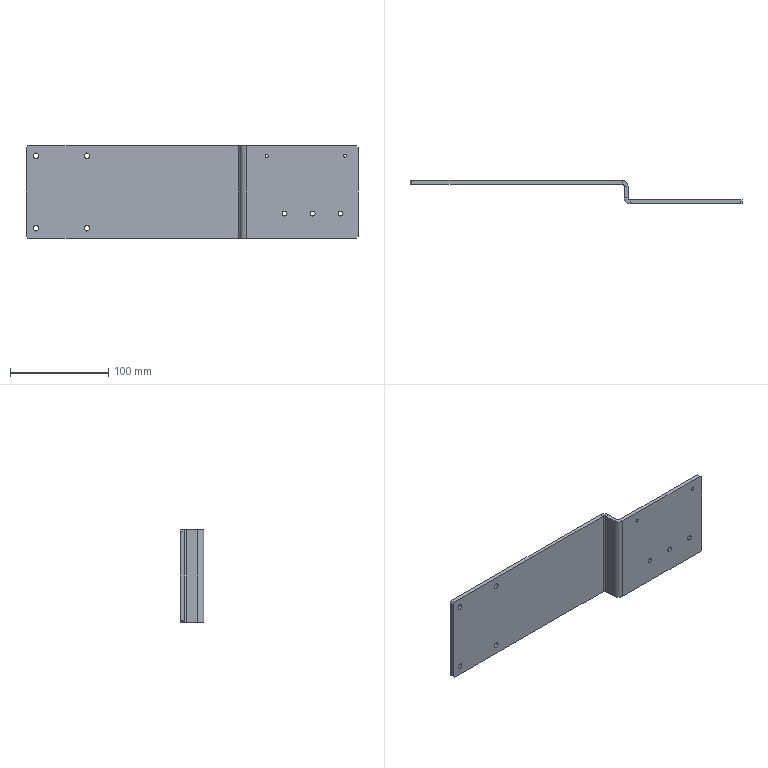Part | NX | features BREP 1 | 1 solid | 44 faces | box 338 x 24 x 94 mm | volume 132601 mm3 | cylinder 22 | plane 22 | commonest cylinder face diameters 5.5 x8 5 x6 3.3 x4 4 x2 12 x2
STEP:
#1=CARTESIAN_POINT('',(325.,-16.,35.35));
#2=VERTEX_POINT('',#1);
#3=CARTESIAN_POINT('',(325.,-20.,35.35));
#4=VERTEX_POINT('',#3);
#5=CARTESIAN_POINT('',(325.,-16.,35.35));
#6=DIRECTION('',(0.,1.,0.));
#7=VECTOR('',#6,1000.);
#8=LINE('',#5,#7);
#9=EDGE_CURVE('',#2,#4,#8,.F.);
#10=ORIENTED_EDGE('',*,*,#9,.T.);
#11=CARTESIAN_POINT('',(325.,-20.,38.65));
#12=VERTEX_POINT('',#11);
#13=CARTESIAN_POINT('',(325.,-20.,37.));
#14=DIRECTION('',(0.,1.,0.));
#15=DIRECTION('',(0.,0.,1.));
#16=AXIS2_PLACEMENT_3D('',#13,#14,#15);
#17=CIRCLE('',#16,1.65);
#18=EDGE_CURVE('',#12,#4,#17,.T.);
#19=ORIENTED_EDGE('',*,*,#18,.F.);
#20=CARTESIAN_POINT('',(325.,-16.,38.65));
#21=VERTEX_POINT('',#20);
#22=CARTESIAN_POINT('',(325.,-16.,38.65));
#23=DIRECTION('',(0.,1.,0.));
#24=VECTOR('',#23,1000.);
#25=LINE('',#22,#24);
#26=EDGE_CURVE('',#21,#12,#25,.F.);
#27=ORIENTED_EDGE('',*,*,#26,.F.);
#28=CARTESIAN_POINT('',(325.,-16.,37.));
#29=DIRECTION('',(0.,1.,0.));
#30=DIRECTION('',(0.,0.,1.));
#31=AXIS2_PLACEMENT_3D('',#28,#29,#30);
#32=CIRCLE('',#31,1.65);
#33=EDGE_CURVE('',#21,#2,#32,.T.);
#34=ORIENTED_EDGE('',*,*,#33,.T.);
#35=EDGE_LOOP('',(#10,#19,#27,#34));
#36=FACE_BOUND('',#35,.T.);
#37=CARTESIAN_POINT('',(325.,-16.,37.));
#38=DIRECTION('',(0.,1.,0.));
#39=DIRECTION('',(0.,0.,1.));
#40=AXIS2_PLACEMENT_3D('',#37,#38,#39);
#41=CYLINDRICAL_SURFACE('',#40,1.65);
#42=ADVANCED_FACE('',(#36),#41,.F.);
#43=CARTESIAN_POINT('',(245.,-16.,35.35));
#44=VERTEX_POINT('',#43);
#45=CARTESIAN_POINT('',(245.,-20.,35.35));
#46=VERTEX_POINT('',#45);
#47=CARTESIAN_POINT('',(245.,-16.,35.35));
#48=DIRECTION('',(0.,1.,0.));
#49=VECTOR('',#48,1000.);
#50=LINE('',#47,#49);
#51=EDGE_CURVE('',#44,#46,#50,.F.);
#52=ORIENTED_EDGE('',*,*,#51,.T.);
#53=CARTESIAN_POINT('',(245.,-20.,38.65));
#54=VERTEX_POINT('',#53);
#55=CARTESIAN_POINT('',(245.,-20.,37.));
#56=DIRECTION('',(0.,1.,0.));
#57=DIRECTION('',(0.,0.,1.));
#58=AXIS2_PLACEMENT_3D('',#55,#56,#57);
#59=CIRCLE('',#58,1.65);
#60=EDGE_CURVE('',#54,#46,#59,.T.);
#61=ORIENTED_EDGE('',*,*,#60,.F.);
#62=CARTESIAN_POINT('',(245.,-16.,38.65));
#63=VERTEX_POINT('',#62);
#64=CARTESIAN_POINT('',(245.,-16.,38.65));
#65=DIRECTION('',(0.,1.,0.));
#66=VECTOR('',#65,1000.);
#67=LINE('',#64,#66);
#68=EDGE_CURVE('',#63,#54,#67,.F.);
#69=ORIENTED_EDGE('',*,*,#68,.F.);
#70=CARTESIAN_POINT('',(245.,-16.,37.));
#71=DIRECTION('',(0.,1.,0.));
#72=DIRECTION('',(0.,0.,1.));
#73=AXIS2_PLACEMENT_3D('',#70,#71,#72);
#74=CIRCLE('',#73,1.65);
#75=EDGE_CURVE('',#63,#44,#74,.T.);
#76=ORIENTED_EDGE('',*,*,#75,.T.);
#77=EDGE_LOOP('',(#52,#61,#69,#76));
#78=FACE_BOUND('',#77,.T.);
#79=CARTESIAN_POINT('',(245.,-16.,37.));
#80=DIRECTION('',(0.,1.,0.));
#81=DIRECTION('',(0.,0.,1.));
#82=AXIS2_PLACEMENT_3D('',#79,#80,#81);
#83=CYLINDRICAL_SURFACE('',#82,1.65);
#84=ADVANCED_FACE('',(#78),#83,.F.);
#85=CARTESIAN_POINT('',(336.,-16.,47.));
#86=VERTEX_POINT('',#85);
#87=CARTESIAN_POINT('',(338.,-16.,45.));
#88=VERTEX_POINT('',#87);
#89=CARTESIAN_POINT('',(277.,-16.,106.));
#90=DIRECTION('',(0.7071,0.,-0.7071));
#91=VECTOR('',#90,1000.);
#92=LINE('',#89,#91);
#93=EDGE_CURVE('',#86,#88,#92,.T.);
#94=ORIENTED_EDGE('',*,*,#93,.F.);
#95=CARTESIAN_POINT('',(336.,-20.,47.));
#96=VERTEX_POINT('',#95);
#97=CARTESIAN_POINT('',(336.,-14.,47.));
#98=DIRECTION('',(0.,1.,0.));
#99=VECTOR('',#98,1000.);
#100=LINE('',#97,#99);
#101=EDGE_CURVE('',#96,#86,#100,.T.);
#102=ORIENTED_EDGE('',*,*,#101,.F.);
#103=CARTESIAN_POINT('',(338.,-20.,45.));
#104=VERTEX_POINT('',#103);
#105=CARTESIAN_POINT('',(338.,-20.,45.));
#106=DIRECTION('',(-0.7071,0.,0.7071));
#107=VECTOR('',#106,1000.);
#108=LINE('',#105,#107);
#109=EDGE_CURVE('',#104,#96,#108,.T.);
#110=ORIENTED_EDGE('',*,*,#109,.F.);
#111=CARTESIAN_POINT('',(338.,-16.,45.));
#112=DIRECTION('',(0.,-1.,0.));
#113=VECTOR('',#112,1000.);
#114=LINE('',#111,#113);
#115=EDGE_CURVE('',#88,#104,#114,.T.);
#116=ORIENTED_EDGE('',*,*,#115,.F.);
#117=EDGE_LOOP('',(#94,#102,#110,#116));
#118=FACE_BOUND('',#117,.T.);
#119=CARTESIAN_POINT('',(338.,-16.,45.));
#120=DIRECTION('',(-0.7071,0.,-0.7071));
#121=DIRECTION('',(0.,-1.,0.));
#122=AXIS2_PLACEMENT_3D('',#119,#120,#121);
#123=PLANE('',#122);
#124=ADVANCED_FACE('',(#118),#123,.F.);
#125=CARTESIAN_POINT('',(338.,-16.,-45.));
#126=VERTEX_POINT('',#125);
#127=CARTESIAN_POINT('',(336.,-16.,-47.));
#128=VERTEX_POINT('',#127);
#129=CARTESIAN_POINT('',(324.,-16.,-59.));
#130=DIRECTION('',(-0.7071,0.,-0.7071));
#131=VECTOR('',#130,1000.);
#132=LINE('',#129,#131);
#133=EDGE_CURVE('',#126,#128,#132,.T.);
#134=ORIENTED_EDGE('',*,*,#133,.F.);
#135=CARTESIAN_POINT('',(338.,-20.,-45.));
#136=VERTEX_POINT('',#135);
#137=CARTESIAN_POINT('',(338.,-16.,-45.));
#138=DIRECTION('',(0.,1.,0.));
#139=VECTOR('',#138,1000.);
#140=LINE('',#137,#139);
#141=EDGE_CURVE('',#136,#126,#140,.T.);
#142=ORIENTED_EDGE('',*,*,#141,.F.);
#143=CARTESIAN_POINT('',(336.,-20.,-47.));
#144=VERTEX_POINT('',#143);
#145=CARTESIAN_POINT('',(336.,-20.,-47.));
#146=DIRECTION('',(0.7071,0.,0.7071));
#147=VECTOR('',#146,1000.);
#148=LINE('',#145,#147);
#149=EDGE_CURVE('',#144,#136,#148,.T.);
#150=ORIENTED_EDGE('',*,*,#149,.F.);
#151=CARTESIAN_POINT('',(336.,-14.,-47.));
#152=DIRECTION('',(0.,-1.,0.));
#153=VECTOR('',#152,1000.);
#154=LINE('',#151,#153);
#155=EDGE_CURVE('',#128,#144,#154,.T.);
#156=ORIENTED_EDGE('',*,*,#155,.F.);
#157=EDGE_LOOP('',(#134,#142,#150,#156));
#158=FACE_BOUND('',#157,.T.);
#159=CARTESIAN_POINT('',(336.,-14.,-47.));
#160=DIRECTION('',(-0.7071,0.,0.7071));
#161=DIRECTION('',(0.,-1.,0.));
#162=AXIS2_PLACEMENT_3D('',#159,#160,#161);
#163=PLANE('',#162);
#164=ADVANCED_FACE('',(#158),#163,.F.);
#165=CARTESIAN_POINT('',(2.,0.,47.));
#166=VERTEX_POINT('',#165);
#167=CARTESIAN_POINT('',(0.,0.,45.));
#168=VERTEX_POINT('',#167);
#169=CARTESIAN_POINT('',(0.,0.,45.));
#170=DIRECTION('',(-0.7071,0.,-0.7071));
#171=VECTOR('',#170,1000.);
#172=LINE('',#169,#171);
#173=EDGE_CURVE('',#166,#168,#172,.T.);
#174=ORIENTED_EDGE('',*,*,#173,.F.);
#175=CARTESIAN_POINT('',(2.,4.,47.));
#176=VERTEX_POINT('',#175);
#177=CARTESIAN_POINT('',(2.,-2.,47.));
#178=DIRECTION('',(0.,-1.,0.));
#179=VECTOR('',#178,1000.);
#180=LINE('',#177,#179);
#181=EDGE_CURVE('',#176,#166,#180,.T.);
#182=ORIENTED_EDGE('',*,*,#181,.F.);
#183=CARTESIAN_POINT('',(0.,4.,45.));
#184=VERTEX_POINT('',#183);
#185=CARTESIAN_POINT('',(1.,4.,46.));
#186=DIRECTION('',(0.7071,0.,0.7071));
#187=VECTOR('',#186,1000.);
#188=LINE('',#185,#187);
#189=EDGE_CURVE('',#184,#176,#188,.T.);
#190=ORIENTED_EDGE('',*,*,#189,.F.);
#191=CARTESIAN_POINT('',(0.,0.,45.));
#192=DIRECTION('',(0.,1.,0.));
#193=VECTOR('',#192,1000.);
#194=LINE('',#191,#193);
#195=EDGE_CURVE('',#168,#184,#194,.T.);
#196=ORIENTED_EDGE('',*,*,#195,.F.);
#197=EDGE_LOOP('',(#174,#182,#190,#196));
#198=FACE_BOUND('',#197,.T.);
#199=CARTESIAN_POINT('',(0.,0.,45.));
#200=DIRECTION('',(0.7071,0.,-0.7071));
#201=DIRECTION('',(0.,1.,0.));
#202=AXIS2_PLACEMENT_3D('',#199,#200,#201);
#203=PLANE('',#202);
#204=ADVANCED_FACE('',(#198),#203,.F.);
#205=CARTESIAN_POINT('',(0.,0.,-45.));
#206=VERTEX_POINT('',#205);
#207=CARTESIAN_POINT('',(2.,0.,-47.));
#208=VERTEX_POINT('',#207);
#209=CARTESIAN_POINT('',(2.,0.,-47.));
#210=DIRECTION('',(0.7071,0.,-0.7071));
#211=VECTOR('',#210,1000.);
#212=LINE('',#209,#211);
#213=EDGE_CURVE('',#206,#208,#212,.T.);
#214=ORIENTED_EDGE('',*,*,#213,.F.);
#215=CARTESIAN_POINT('',(0.,4.,-45.));
#216=VERTEX_POINT('',#215);
#217=CARTESIAN_POINT('',(0.,0.,-45.));
#218=DIRECTION('',(0.,-1.,0.));
#219=VECTOR('',#218,1000.);
#220=LINE('',#217,#219);
#221=EDGE_CURVE('',#216,#206,#220,.T.);
#222=ORIENTED_EDGE('',*,*,#221,.F.);
#223=CARTESIAN_POINT('',(2.,4.,-47.));
#224=VERTEX_POINT('',#223);
#225=CARTESIAN_POINT('',(-46.,4.,1.));
#226=DIRECTION('',(-0.7071,0.,0.7071));
#227=VECTOR('',#226,1000.);
#228=LINE('',#225,#227);
#229=EDGE_CURVE('',#224,#216,#228,.T.);
#230=ORIENTED_EDGE('',*,*,#229,.F.);
#231=CARTESIAN_POINT('',(2.,4.,-47.));
#232=DIRECTION('',(0.,1.,0.));
#233=VECTOR('',#232,1000.);
#234=LINE('',#231,#233);
#235=EDGE_CURVE('',#208,#224,#234,.T.);
#236=ORIENTED_EDGE('',*,*,#235,.F.);
#237=EDGE_LOOP('',(#214,#222,#230,#236));
#238=FACE_BOUND('',#237,.T.);
#239=CARTESIAN_POINT('',(2.,-14.,-47.));
#240=DIRECTION('',(-0.7071,0.,-0.7071));
#241=DIRECTION('',(0.,-1.,0.));
#242=AXIS2_PLACEMENT_3D('',#239,#240,#241);
#243=PLANE('',#242);
#244=ADVANCED_FACE('',(#238),#243,.T.);
#245=CARTESIAN_POINT('',(263.3,-16.,-24.5));
#246=VERTEX_POINT('',#245);
#247=CARTESIAN_POINT('',(263.3,-20.,-24.5));
#248=VERTEX_POINT('',#247);
#249=CARTESIAN_POINT('',(263.3,-16.,-24.5));
#250=DIRECTION('',(0.,1.,0.));
#251=VECTOR('',#250,1000.);
#252=LINE('',#249,#251);
#253=EDGE_CURVE('',#246,#248,#252,.F.);
#254=ORIENTED_EDGE('',*,*,#253,.T.);
#255=CARTESIAN_POINT('',(263.3,-20.,-19.5));
#256=VERTEX_POINT('',#255);
#257=CARTESIAN_POINT('',(263.3,-20.,-22.));
#258=DIRECTION('',(0.,1.,0.));
#259=DIRECTION('',(0.,0.,1.));
#260=AXIS2_PLACEMENT_3D('',#257,#258,#259);
#261=CIRCLE('',#260,2.5);
#262=EDGE_CURVE('',#256,#248,#261,.T.);
#263=ORIENTED_EDGE('',*,*,#262,.F.);
#264=CARTESIAN_POINT('',(263.3,-16.,-19.5));
#265=VERTEX_POINT('',#264);
#266=CARTESIAN_POINT('',(263.3,-16.,-19.5));
#267=DIRECTION('',(0.,1.,0.));
#268=VECTOR('',#267,1000.);
#269=LINE('',#266,#268);
#270=EDGE_CURVE('',#265,#256,#269,.F.);
#271=ORIENTED_EDGE('',*,*,#270,.F.);
#272=CARTESIAN_POINT('',(263.3,-16.,-22.));
#273=DIRECTION('',(0.,1.,0.));
#274=DIRECTION('',(0.,0.,1.));
#275=AXIS2_PLACEMENT_3D('',#272,#273,#274);
#276=CIRCLE('',#275,2.5);
#277=EDGE_CURVE('',#265,#246,#276,.T.);
#278=ORIENTED_EDGE('',*,*,#277,.T.);
#279=EDGE_LOOP('',(#254,#263,#271,#278));
#280=FACE_BOUND('',#279,.T.);
#281=CARTESIAN_POINT('',(263.3,-16.,-22.));
#282=DIRECTION('',(0.,1.,0.));
#283=DIRECTION('',(0.,0.,1.));
#284=AXIS2_PLACEMENT_3D('',#281,#282,#283);
#285=CYLINDRICAL_SURFACE('',#284,2.5);
#286=ADVANCED_FACE('',(#280),#285,.F.);
#287=CARTESIAN_POINT('',(291.8,-16.,-24.5));
#288=VERTEX_POINT('',#287);
#289=CARTESIAN_POINT('',(291.8,-20.,-24.5));
#290=VERTEX_POINT('',#289);
#291=CARTESIAN_POINT('',(291.8,-16.,-24.5));
#292=DIRECTION('',(0.,1.,0.));
#293=VECTOR('',#292,1000.);
#294=LINE('',#291,#293);
#295=EDGE_CURVE('',#288,#290,#294,.F.);
#296=ORIENTED_EDGE('',*,*,#295,.T.);
#297=CARTESIAN_POINT('',(291.8,-20.,-19.5));
#298=VERTEX_POINT('',#297);
#299=CARTESIAN_POINT('',(291.8,-20.,-22.));
#300=DIRECTION('',(0.,1.,0.));
#301=DIRECTION('',(0.,0.,1.));
#302=AXIS2_PLACEMENT_3D('',#299,#300,#301);
#303=CIRCLE('',#302,2.5);
#304=EDGE_CURVE('',#298,#290,#303,.T.);
#305=ORIENTED_EDGE('',*,*,#304,.F.);
#306=CARTESIAN_POINT('',(291.8,-16.,-19.5));
#307=VERTEX_POINT('',#306);
#308=CARTESIAN_POINT('',(291.8,-16.,-19.5));
#309=DIRECTION('',(0.,1.,0.));
#310=VECTOR('',#309,1000.);
#311=LINE('',#308,#310);
#312=EDGE_CURVE('',#307,#298,#311,.F.);
#313=ORIENTED_EDGE('',*,*,#312,.F.);
#314=CARTESIAN_POINT('',(291.8,-16.,-22.));
#315=DIRECTION('',(0.,1.,0.));
#316=DIRECTION('',(0.,0.,1.));
#317=AXIS2_PLACEMENT_3D('',#314,#315,#316);
#318=CIRCLE('',#317,2.5);
#319=EDGE_CURVE('',#307,#288,#318,.T.);
#320=ORIENTED_EDGE('',*,*,#319,.T.);
#321=EDGE_LOOP('',(#296,#305,#313,#320));
#322=FACE_BOUND('',#321,.T.);
#323=CARTESIAN_POINT('',(291.8,-16.,-22.));
#324=DIRECTION('',(0.,1.,0.));
#325=DIRECTION('',(0.,0.,1.));
#326=AXIS2_PLACEMENT_3D('',#323,#324,#325);
#327=CYLINDRICAL_SURFACE('',#326,2.5);
#328=ADVANCED_FACE('',(#322),#327,.F.);
#329=CARTESIAN_POINT('',(320.3,-16.,-24.5));
#330=VERTEX_POINT('',#329);
#331=CARTESIAN_POINT('',(320.3,-20.,-24.5));
#332=VERTEX_POINT('',#331);
#333=CARTESIAN_POINT('',(320.3,-16.,-24.5));
#334=DIRECTION('',(0.,1.,0.));
#335=VECTOR('',#334,1000.);
#336=LINE('',#333,#335);
#337=EDGE_CURVE('',#330,#332,#336,.F.);
#338=ORIENTED_EDGE('',*,*,#337,.T.);
#339=CARTESIAN_POINT('',(320.3,-20.,-19.5));
#340=VERTEX_POINT('',#339);
#341=CARTESIAN_POINT('',(320.3,-20.,-22.));
#342=DIRECTION('',(0.,1.,0.));
#343=DIRECTION('',(0.,0.,1.));
#344=AXIS2_PLACEMENT_3D('',#341,#342,#343);
#345=CIRCLE('',#344,2.5);
#346=EDGE_CURVE('',#340,#332,#345,.T.);
#347=ORIENTED_EDGE('',*,*,#346,.F.);
#348=CARTESIAN_POINT('',(320.3,-16.,-19.5));
#349=VERTEX_POINT('',#348);
#350=CARTESIAN_POINT('',(320.3,-16.,-19.5));
#351=DIRECTION('',(0.,1.,0.));
#352=VECTOR('',#351,1000.);
#353=LINE('',#350,#352);
#354=EDGE_CURVE('',#349,#340,#353,.F.);
#355=ORIENTED_EDGE('',*,*,#354,.F.);
#356=CARTESIAN_POINT('',(320.3,-16.,-22.));
#357=DIRECTION('',(0.,1.,0.));
#358=DIRECTION('',(0.,0.,1.));
#359=AXIS2_PLACEMENT_3D('',#356,#357,#358);
#360=CIRCLE('',#359,2.5);
#361=EDGE_CURVE('',#349,#330,#360,.T.);
#362=ORIENTED_EDGE('',*,*,#361,.T.);
#363=EDGE_LOOP('',(#338,#347,#355,#362));
#364=FACE_BOUND('',#363,.T.);
#365=CARTESIAN_POINT('',(320.3,-16.,-22.));
#366=DIRECTION('',(0.,1.,0.));
#367=DIRECTION('',(0.,0.,1.));
#368=AXIS2_PLACEMENT_3D('',#365,#366,#367);
#369=CYLINDRICAL_SURFACE('',#368,2.5);
#370=ADVANCED_FACE('',(#364),#369,.F.);
#371=CARTESIAN_POINT('',(10.,4.,-39.75));
#372=VERTEX_POINT('',#371);
#373=CARTESIAN_POINT('',(10.,0.,-39.75));
#374=VERTEX_POINT('',#373);
#375=CARTESIAN_POINT('',(10.,4.,-39.75));
#376=DIRECTION('',(0.,1.,0.));
#377=VECTOR('',#376,1000.);
#378=LINE('',#375,#377);
#379=EDGE_CURVE('',#372,#374,#378,.F.);
#380=ORIENTED_EDGE('',*,*,#379,.T.);
#381=CARTESIAN_POINT('',(10.,0.,-34.25));
#382=VERTEX_POINT('',#381);
#383=CARTESIAN_POINT('',(10.,0.,-37.));
#384=DIRECTION('',(0.,1.,0.));
#385=DIRECTION('',(0.,0.,1.));
#386=AXIS2_PLACEMENT_3D('',#383,#384,#385);
#387=CIRCLE('',#386,2.75);
#388=EDGE_CURVE('',#382,#374,#387,.T.);
#389=ORIENTED_EDGE('',*,*,#388,.F.);
#390=CARTESIAN_POINT('',(10.,4.,-34.25));
#391=VERTEX_POINT('',#390);
#392=CARTESIAN_POINT('',(10.,4.,-34.25));
#393=DIRECTION('',(0.,1.,0.));
#394=VECTOR('',#393,1000.);
#395=LINE('',#392,#394);
#396=EDGE_CURVE('',#391,#382,#395,.F.);
#397=ORIENTED_EDGE('',*,*,#396,.F.);
#398=CARTESIAN_POINT('',(10.,4.,-37.));
#399=DIRECTION('',(0.,1.,0.));
#400=DIRECTION('',(0.,0.,1.));
#401=AXIS2_PLACEMENT_3D('',#398,#399,#400);
#402=CIRCLE('',#401,2.75);
#403=EDGE_CURVE('',#391,#372,#402,.T.);
#404=ORIENTED_EDGE('',*,*,#403,.T.);
#405=EDGE_LOOP('',(#380,#389,#397,#404));
#406=FACE_BOUND('',#405,.T.);
#407=CARTESIAN_POINT('',(10.,4.,-37.));
#408=DIRECTION('',(0.,1.,0.));
#409=DIRECTION('',(0.,0.,1.));
#410=AXIS2_PLACEMENT_3D('',#407,#408,#409);
#411=CYLINDRICAL_SURFACE('',#410,2.75);
#412=ADVANCED_FACE('',(#406),#411,.F.);
#413=CARTESIAN_POINT('',(62.,4.,-39.75));
#414=VERTEX_POINT('',#413);
#415=CARTESIAN_POINT('',(62.,0.,-39.75));
#416=VERTEX_POINT('',#415);
#417=CARTESIAN_POINT('',(62.,4.,-39.75));
#418=DIRECTION('',(0.,1.,0.));
#419=VECTOR('',#418,1000.);
#420=LINE('',#417,#419);
#421=EDGE_CURVE('',#414,#416,#420,.F.);
#422=ORIENTED_EDGE('',*,*,#421,.T.);
#423=CARTESIAN_POINT('',(62.,0.,-34.25));
#424=VERTEX_POINT('',#423);
#425=CARTESIAN_POINT('',(62.,0.,-37.));
#426=DIRECTION('',(0.,1.,0.));
#427=DIRECTION('',(0.,0.,1.));
#428=AXIS2_PLACEMENT_3D('',#425,#426,#427);
#429=CIRCLE('',#428,2.75);
#430=EDGE_CURVE('',#424,#416,#429,.T.);
#431=ORIENTED_EDGE('',*,*,#430,.F.);
#432=CARTESIAN_POINT('',(62.,4.,-34.25));
#433=VERTEX_POINT('',#432);
#434=CARTESIAN_POINT('',(62.,4.,-34.25));
#435=DIRECTION('',(0.,1.,0.));
#436=VECTOR('',#435,1000.);
#437=LINE('',#434,#436);
#438=EDGE_CURVE('',#433,#424,#437,.F.);
#439=ORIENTED_EDGE('',*,*,#438,.F.);
#440=CARTESIAN_POINT('',(62.,4.,-37.));
#441=DIRECTION('',(0.,1.,0.));
#442=DIRECTION('',(0.,0.,1.));
#443=AXIS2_PLACEMENT_3D('',#440,#441,#442);
#444=CIRCLE('',#443,2.75);
#445=EDGE_CURVE('',#433,#414,#444,.T.);
#446=ORIENTED_EDGE('',*,*,#445,.T.);
#447=EDGE_LOOP('',(#422,#431,#439,#446));
#448=FACE_BOUND('',#447,.T.);
#449=CARTESIAN_POINT('',(62.,4.,-37.));
#450=DIRECTION('',(0.,1.,0.));
#451=DIRECTION('',(0.,0.,1.));
#452=AXIS2_PLACEMENT_3D('',#449,#450,#451);
#453=CYLINDRICAL_SURFACE('',#452,2.75);
#454=ADVANCED_FACE('',(#448),#453,.F.);
#455=CARTESIAN_POINT('',(10.,4.,34.25));
#456=VERTEX_POINT('',#455);
#457=CARTESIAN_POINT('',(10.,0.,34.25));
#458=VERTEX_POINT('',#457);
#459=CARTESIAN_POINT('',(10.,4.,34.25));
#460=DIRECTION('',(0.,1.,0.));
#461=VECTOR('',#460,1000.);
#462=LINE('',#459,#461);
#463=EDGE_CURVE('',#456,#458,#462,.F.);
#464=ORIENTED_EDGE('',*,*,#463,.T.);
#465=CARTESIAN_POINT('',(10.,0.,39.75));
#466=VERTEX_POINT('',#465);
#467=CARTESIAN_POINT('',(10.,0.,37.));
#468=DIRECTION('',(0.,1.,0.));
#469=DIRECTION('',(0.,0.,1.));
#470=AXIS2_PLACEMENT_3D('',#467,#468,#469);
#471=CIRCLE('',#470,2.75);
#472=EDGE_CURVE('',#466,#458,#471,.T.);
#473=ORIENTED_EDGE('',*,*,#472,.F.);
#474=CARTESIAN_POINT('',(10.,4.,39.75));
#475=VERTEX_POINT('',#474);
#476=CARTESIAN_POINT('',(10.,4.,39.75));
#477=DIRECTION('',(0.,1.,0.));
#478=VECTOR('',#477,1000.);
#479=LINE('',#476,#478);
#480=EDGE_CURVE('',#475,#466,#479,.F.);
#481=ORIENTED_EDGE('',*,*,#480,.F.);
#482=CARTESIAN_POINT('',(10.,4.,37.));
#483=DIRECTION('',(0.,1.,0.));
#484=DIRECTION('',(0.,0.,1.));
#485=AXIS2_PLACEMENT_3D('',#482,#483,#484);
#486=CIRCLE('',#485,2.75);
#487=EDGE_CURVE('',#475,#456,#486,.T.);
#488=ORIENTED_EDGE('',*,*,#487,.T.);
#489=EDGE_LOOP('',(#464,#473,#481,#488));
#490=FACE_BOUND('',#489,.T.);
#491=CARTESIAN_POINT('',(10.,4.,37.));
#492=DIRECTION('',(0.,1.,0.));
#493=DIRECTION('',(0.,0.,1.));
#494=AXIS2_PLACEMENT_3D('',#491,#492,#493);
#495=CYLINDRICAL_SURFACE('',#494,2.75);
#496=ADVANCED_FACE('',(#490),#495,.F.);
#497=CARTESIAN_POINT('',(62.,4.,34.25));
#498=VERTEX_POINT('',#497);
#499=CARTESIAN_POINT('',(62.,0.,34.25));
#500=VERTEX_POINT('',#499);
#501=CARTESIAN_POINT('',(62.,4.,34.25));
#502=DIRECTION('',(0.,1.,0.));
#503=VECTOR('',#502,1000.);
#504=LINE('',#501,#503);
#505=EDGE_CURVE('',#498,#500,#504,.F.);
#506=ORIENTED_EDGE('',*,*,#505,.T.);
#507=CARTESIAN_POINT('',(62.,0.,39.75));
#508=VERTEX_POINT('',#507);
#509=CARTESIAN_POINT('',(62.,0.,37.));
#510=DIRECTION('',(0.,1.,0.));
#511=DIRECTION('',(0.,0.,1.));
#512=AXIS2_PLACEMENT_3D('',#509,#510,#511);
#513=CIRCLE('',#512,2.75);
#514=EDGE_CURVE('',#508,#500,#513,.T.);
#515=ORIENTED_EDGE('',*,*,#514,.F.);
#516=CARTESIAN_POINT('',(62.,4.,39.75));
#517=VERTEX_POINT('',#516);
#518=CARTESIAN_POINT('',(62.,4.,39.75));
#519=DIRECTION('',(0.,1.,0.));
#520=VECTOR('',#519,1000.);
#521=LINE('',#518,#520);
#522=EDGE_CURVE('',#517,#508,#521,.F.);
#523=ORIENTED_EDGE('',*,*,#522,.F.);
#524=CARTESIAN_POINT('',(62.,4.,37.));
#525=DIRECTION('',(0.,1.,0.));
#526=DIRECTION('',(0.,0.,1.));
#527=AXIS2_PLACEMENT_3D('',#524,#525,#526);
#528=CIRCLE('',#527,2.75);
#529=EDGE_CURVE('',#517,#498,#528,.T.);
#530=ORIENTED_EDGE('',*,*,#529,.T.);
#531=EDGE_LOOP('',(#506,#515,#523,#530));
#532=FACE_BOUND('',#531,.T.);
#533=CARTESIAN_POINT('',(62.,4.,37.));
#534=DIRECTION('',(0.,1.,0.));
#535=DIRECTION('',(0.,0.,1.));
#536=AXIS2_PLACEMENT_3D('',#533,#534,#535);
#537=CYLINDRICAL_SURFACE('',#536,2.75);
#538=ADVANCED_FACE('',(#532),#537,.F.);
#539=CARTESIAN_POINT('',(216.,0.,-47.));
#540=VERTEX_POINT('',#539);
#541=CARTESIAN_POINT('',(0.,0.,-47.));
#542=DIRECTION('',(1.,0.,0.));
#543=VECTOR('',#542,1000.);
#544=LINE('',#541,#543);
#545=EDGE_CURVE('',#208,#540,#544,.T.);
#546=ORIENTED_EDGE('',*,*,#545,.F.);
#547=ORIENTED_EDGE('',*,*,#235,.T.);
#548=CARTESIAN_POINT('',(216.,4.,-47.));
#549=VERTEX_POINT('',#548);
#550=CARTESIAN_POINT('',(0.,4.,-47.));
#551=DIRECTION('',(1.,0.,0.));
#552=VECTOR('',#551,1000.);
#553=LINE('',#550,#552);
#554=EDGE_CURVE('',#224,#549,#553,.T.);
#555=ORIENTED_EDGE('',*,*,#554,.T.);
#556=CARTESIAN_POINT('',(216.,4.,-47.));
#557=DIRECTION('',(0.,-1.,0.));
#558=VECTOR('',#557,1000.);
#559=LINE('',#556,#558);
#560=EDGE_CURVE('',#549,#540,#559,.T.);
#561=ORIENTED_EDGE('',*,*,#560,.T.);
#562=EDGE_LOOP('',(#546,#547,#555,#561));
#563=FACE_BOUND('',#562,.T.);
#564=CARTESIAN_POINT('',(224.,-14.,-47.));
#565=DIRECTION('',(0.,0.,1.));
#566=DIRECTION('',(1.,0.,0.));
#567=AXIS2_PLACEMENT_3D('',#564,#565,#566);
#568=PLANE('',#567);
#569=ADVANCED_FACE('',(#563),#568,.F.);
#570=CARTESIAN_POINT('',(224.,-20.,47.));
#571=VERTEX_POINT('',#570);
#572=CARTESIAN_POINT('',(218.,-20.,47.));
#573=DIRECTION('',(1.,0.,0.));
#574=VECTOR('',#573,1000.);
#575=LINE('',#572,#574);
#576=EDGE_CURVE('',#571,#96,#575,.T.);
#577=ORIENTED_EDGE('',*,*,#576,.T.);
#578=ORIENTED_EDGE('',*,*,#101,.T.);
#579=CARTESIAN_POINT('',(224.,-16.,47.));
#580=VERTEX_POINT('',#579);
#581=CARTESIAN_POINT('',(218.,-16.,47.));
#582=DIRECTION('',(1.,0.,0.));
#583=VECTOR('',#582,1000.);
#584=LINE('',#581,#583);
#585=EDGE_CURVE('',#580,#86,#584,.T.);
#586=ORIENTED_EDGE('',*,*,#585,.F.);
#587=CARTESIAN_POINT('',(224.,-16.,47.));
#588=DIRECTION('',(0.,-1.,0.));
#589=VECTOR('',#588,1000.);
#590=LINE('',#587,#589);
#591=EDGE_CURVE('',#580,#571,#590,.T.);
#592=ORIENTED_EDGE('',*,*,#591,.T.);
#593=EDGE_LOOP('',(#577,#578,#586,#592));
#594=FACE_BOUND('',#593,.T.);
#595=CARTESIAN_POINT('',(224.,-14.,47.));
#596=DIRECTION('',(0.,0.,1.));
#597=DIRECTION('',(1.,0.,0.));
#598=AXIS2_PLACEMENT_3D('',#595,#596,#597);
#599=PLANE('',#598);
#600=ADVANCED_FACE('',(#594),#599,.T.);
#601=CARTESIAN_POINT('',(218.,-14.,-47.));
#602=VERTEX_POINT('',#601);
#603=CARTESIAN_POINT('',(224.,-20.,-47.));
#604=VERTEX_POINT('',#603);
#605=CARTESIAN_POINT('',(224.,-14.,-47.));
#606=DIRECTION('',(0.,0.,1.));
#607=DIRECTION('',(-1.,0.,0.));
#608=AXIS2_PLACEMENT_3D('',#605,#606,#607);
#609=CIRCLE('',#608,6.);
#610=EDGE_CURVE('',#602,#604,#609,.T.);
#611=ORIENTED_EDGE('',*,*,#610,.T.);
#612=CARTESIAN_POINT('',(224.,-20.,47.));
#613=DIRECTION('',(0.,0.,-1.));
#614=VECTOR('',#613,1000.);
#615=LINE('',#612,#614);
#616=EDGE_CURVE('',#571,#604,#615,.T.);
#617=ORIENTED_EDGE('',*,*,#616,.F.);
#618=CARTESIAN_POINT('',(218.,-14.,47.));
#619=VERTEX_POINT('',#618);
#620=CARTESIAN_POINT('',(224.,-14.,47.));
#621=DIRECTION('',(0.,0.,1.));
#622=DIRECTION('',(-1.,0.,0.));
#623=AXIS2_PLACEMENT_3D('',#620,#621,#622);
#624=CIRCLE('',#623,6.);
#625=EDGE_CURVE('',#619,#571,#624,.T.);
#626=ORIENTED_EDGE('',*,*,#625,.F.);
#627=CARTESIAN_POINT('',(218.,-14.,47.));
#628=DIRECTION('',(0.,0.,-1.));
#629=VECTOR('',#628,1000.);
#630=LINE('',#627,#629);
#631=EDGE_CURVE('',#619,#602,#630,.T.);
#632=ORIENTED_EDGE('',*,*,#631,.T.);
#633=EDGE_LOOP('',(#611,#617,#626,#632));
#634=FACE_BOUND('',#633,.T.);
#635=CARTESIAN_POINT('',(224.,-14.,47.));
#636=DIRECTION('',(0.,0.,-1.));
#637=DIRECTION('',(-1.,0.,0.));
#638=AXIS2_PLACEMENT_3D('',#635,#636,#637);
#639=CYLINDRICAL_SURFACE('',#638,6.);
#640=ADVANCED_FACE('',(#634),#639,.T.);
#641=CARTESIAN_POINT('',(218.,-2.,-47.));
#642=VERTEX_POINT('',#641);
#643=CARTESIAN_POINT('',(218.,0.,-47.));
#644=DIRECTION('',(0.,-1.,0.));
#645=VECTOR('',#644,1000.);
#646=LINE('',#643,#645);
#647=EDGE_CURVE('',#642,#602,#646,.T.);
#648=ORIENTED_EDGE('',*,*,#647,.T.);
#649=ORIENTED_EDGE('',*,*,#631,.F.);
#650=CARTESIAN_POINT('',(218.,-2.,47.));
#651=VERTEX_POINT('',#650);
#652=CARTESIAN_POINT('',(218.,0.,47.));
#653=DIRECTION('',(0.,-1.,0.));
#654=VECTOR('',#653,1000.);
#655=LINE('',#652,#654);
#656=EDGE_CURVE('',#651,#619,#655,.T.);
#657=ORIENTED_EDGE('',*,*,#656,.F.);
#658=CARTESIAN_POINT('',(218.,-2.,47.));
#659=DIRECTION('',(0.,0.,-1.));
#660=VECTOR('',#659,1000.);
#661=LINE('',#658,#660);
#662=EDGE_CURVE('',#651,#642,#661,.T.);
#663=ORIENTED_EDGE('',*,*,#662,.T.);
#664=EDGE_LOOP('',(#648,#649,#657,#663));
#665=FACE_BOUND('',#664,.T.);
#666=CARTESIAN_POINT('',(218.,0.,47.));
#667=DIRECTION('',(1.,0.,0.));
#668=DIRECTION('',(0.,0.,-1.));
#669=AXIS2_PLACEMENT_3D('',#666,#667,#668);
#670=PLANE('',#669);
#671=ADVANCED_FACE('',(#665),#670,.F.);
#672=CARTESIAN_POINT('',(216.,-2.,-47.));
#673=DIRECTION('',(0.,0.,-1.));
#674=DIRECTION('',(1.,0.,0.));
#675=AXIS2_PLACEMENT_3D('',#672,#673,#674);
#676=CIRCLE('',#675,2.);
#677=EDGE_CURVE('',#540,#642,#676,.T.);
#678=ORIENTED_EDGE('',*,*,#677,.T.);
#679=ORIENTED_EDGE('',*,*,#662,.F.);
#680=CARTESIAN_POINT('',(216.,0.,47.));
#681=VERTEX_POINT('',#680);
#682=CARTESIAN_POINT('',(216.,-2.,47.));
#683=DIRECTION('',(0.,0.,-1.));
#684=DIRECTION('',(1.,0.,0.));
#685=AXIS2_PLACEMENT_3D('',#682,#683,#684);
#686=CIRCLE('',#685,2.);
#687=EDGE_CURVE('',#681,#651,#686,.T.);
#688=ORIENTED_EDGE('',*,*,#687,.F.);
#689=CARTESIAN_POINT('',(216.,0.,47.));
#690=DIRECTION('',(0.,0.,-1.));
#691=VECTOR('',#690,1000.);
#692=LINE('',#689,#691);
#693=EDGE_CURVE('',#681,#540,#692,.T.);
#694=ORIENTED_EDGE('',*,*,#693,.T.);
#695=EDGE_LOOP('',(#678,#679,#688,#694));
#696=FACE_BOUND('',#695,.T.);
#697=CARTESIAN_POINT('',(216.,-2.,47.));
#698=DIRECTION('',(0.,0.,-1.));
#699=DIRECTION('',(-1.,0.,0.));
#700=AXIS2_PLACEMENT_3D('',#697,#698,#699);
#701=CYLINDRICAL_SURFACE('',#700,2.);
#702=ADVANCED_FACE('',(#696),#701,.F.);
#703=CARTESIAN_POINT('',(0.,0.,47.));
#704=DIRECTION('',(0.,0.,-1.));
#705=VECTOR('',#704,1000.);
#706=LINE('',#703,#705);
#707=EDGE_CURVE('',#168,#206,#706,.T.);
#708=ORIENTED_EDGE('',*,*,#707,.T.);
#709=ORIENTED_EDGE('',*,*,#213,.T.);
#710=ORIENTED_EDGE('',*,*,#545,.T.);
#711=ORIENTED_EDGE('',*,*,#693,.F.);
#712=CARTESIAN_POINT('',(0.,0.,47.));
#713=DIRECTION('',(1.,0.,0.));
#714=VECTOR('',#713,1000.);
#715=LINE('',#712,#714);
#716=EDGE_CURVE('',#166,#681,#715,.T.);
#717=ORIENTED_EDGE('',*,*,#716,.F.);
#718=ORIENTED_EDGE('',*,*,#173,.T.);
#719=EDGE_LOOP('',(#708,#709,#710,#711,#717,#718));
#720=FACE_BOUND('',#719,.T.);
#721=ORIENTED_EDGE('',*,*,#514,.T.);
#722=CARTESIAN_POINT('',(62.,0.,37.));
#723=DIRECTION('',(0.,1.,0.));
#724=DIRECTION('',(0.,0.,1.));
#725=AXIS2_PLACEMENT_3D('',#722,#723,#724);
#726=CIRCLE('',#725,2.75);
#727=EDGE_CURVE('',#500,#508,#726,.T.);
#728=ORIENTED_EDGE('',*,*,#727,.T.);
#729=EDGE_LOOP('',(#721,#728));
#730=FACE_BOUND('',#729,.T.);
#731=ORIENTED_EDGE('',*,*,#472,.T.);
#732=CARTESIAN_POINT('',(10.,0.,37.));
#733=DIRECTION('',(0.,1.,0.));
#734=DIRECTION('',(0.,0.,1.));
#735=AXIS2_PLACEMENT_3D('',#732,#733,#734);
#736=CIRCLE('',#735,2.75);
#737=EDGE_CURVE('',#458,#466,#736,.T.);
#738=ORIENTED_EDGE('',*,*,#737,.T.);
#739=EDGE_LOOP('',(#731,#738));
#740=FACE_BOUND('',#739,.T.);
#741=ORIENTED_EDGE('',*,*,#430,.T.);
#742=CARTESIAN_POINT('',(62.,0.,-37.));
#743=DIRECTION('',(0.,1.,0.));
#744=DIRECTION('',(0.,0.,1.));
#745=AXIS2_PLACEMENT_3D('',#742,#743,#744);
#746=CIRCLE('',#745,2.75);
#747=EDGE_CURVE('',#416,#424,#746,.T.);
#748=ORIENTED_EDGE('',*,*,#747,.T.);
#749=EDGE_LOOP('',(#741,#748));
#750=FACE_BOUND('',#749,.T.);
#751=ORIENTED_EDGE('',*,*,#388,.T.);
#752=CARTESIAN_POINT('',(10.,0.,-37.));
#753=DIRECTION('',(0.,1.,0.));
#754=DIRECTION('',(0.,0.,1.));
#755=AXIS2_PLACEMENT_3D('',#752,#753,#754);
#756=CIRCLE('',#755,2.75);
#757=EDGE_CURVE('',#374,#382,#756,.T.);
#758=ORIENTED_EDGE('',*,*,#757,.T.);
#759=EDGE_LOOP('',(#751,#758));
#760=FACE_BOUND('',#759,.T.);
#761=CARTESIAN_POINT('',(0.,0.,47.));
#762=DIRECTION('',(0.,1.,0.));
#763=DIRECTION('',(0.,0.,1.));
#764=AXIS2_PLACEMENT_3D('',#761,#762,#763);
#765=PLANE('',#764);
#766=ADVANCED_FACE('',(#720,#730,#740,#750,#760),#765,.F.);
#767=CARTESIAN_POINT('',(0.,4.,47.));
#768=DIRECTION('',(0.,0.,-1.));
#769=VECTOR('',#768,1000.);
#770=LINE('',#767,#769);
#771=EDGE_CURVE('',#184,#216,#770,.T.);
#772=ORIENTED_EDGE('',*,*,#771,.T.);
#773=ORIENTED_EDGE('',*,*,#221,.T.);
#774=ORIENTED_EDGE('',*,*,#707,.F.);
#775=ORIENTED_EDGE('',*,*,#195,.T.);
#776=EDGE_LOOP('',(#772,#773,#774,#775));
#777=FACE_BOUND('',#776,.T.);
#778=CARTESIAN_POINT('',(0.,0.,47.));
#779=DIRECTION('',(-1.,0.,0.));
#780=DIRECTION('',(0.,0.,1.));
#781=AXIS2_PLACEMENT_3D('',#778,#779,#780);
#782=PLANE('',#781);
#783=ADVANCED_FACE('',(#777),#782,.T.);
#784=ORIENTED_EDGE('',*,*,#554,.F.);
#785=ORIENTED_EDGE('',*,*,#229,.T.);
#786=ORIENTED_EDGE('',*,*,#771,.F.);
#787=ORIENTED_EDGE('',*,*,#189,.T.);
#788=CARTESIAN_POINT('',(216.,4.,47.));
#789=VERTEX_POINT('',#788);
#790=CARTESIAN_POINT('',(0.,4.,47.));
#791=DIRECTION('',(1.,0.,0.));
#792=VECTOR('',#791,1000.);
#793=LINE('',#790,#792);
#794=EDGE_CURVE('',#176,#789,#793,.T.);
#795=ORIENTED_EDGE('',*,*,#794,.T.);
#796=CARTESIAN_POINT('',(216.,4.,47.));
#797=DIRECTION('',(0.,0.,-1.));
#798=VECTOR('',#797,1000.);
#799=LINE('',#796,#798);
#800=EDGE_CURVE('',#789,#549,#799,.T.);
#801=ORIENTED_EDGE('',*,*,#800,.T.);
#802=EDGE_LOOP('',(#784,#785,#786,#787,#795,#801));
#803=FACE_BOUND('',#802,.T.);
#804=ORIENTED_EDGE('',*,*,#529,.F.);
#805=CARTESIAN_POINT('',(62.,4.,37.));
#806=DIRECTION('',(0.,1.,0.));
#807=DIRECTION('',(0.,0.,1.));
#808=AXIS2_PLACEMENT_3D('',#805,#806,#807);
#809=CIRCLE('',#808,2.75);
#810=EDGE_CURVE('',#498,#517,#809,.T.);
#811=ORIENTED_EDGE('',*,*,#810,.F.);
#812=EDGE_LOOP('',(#804,#811));
#813=FACE_BOUND('',#812,.T.);
#814=ORIENTED_EDGE('',*,*,#487,.F.);
#815=CARTESIAN_POINT('',(10.,4.,37.));
#816=DIRECTION('',(0.,1.,0.));
#817=DIRECTION('',(0.,0.,1.));
#818=AXIS2_PLACEMENT_3D('',#815,#816,#817);
#819=CIRCLE('',#818,2.75);
#820=EDGE_CURVE('',#456,#475,#819,.T.);
#821=ORIENTED_EDGE('',*,*,#820,.F.);
#822=EDGE_LOOP('',(#814,#821));
#823=FACE_BOUND('',#822,.T.);
#824=ORIENTED_EDGE('',*,*,#445,.F.);
#825=CARTESIAN_POINT('',(62.,4.,-37.));
#826=DIRECTION('',(0.,1.,0.));
#827=DIRECTION('',(0.,0.,1.));
#828=AXIS2_PLACEMENT_3D('',#825,#826,#827);
#829=CIRCLE('',#828,2.75);
#830=EDGE_CURVE('',#414,#433,#829,.T.);
#831=ORIENTED_EDGE('',*,*,#830,.F.);
#832=EDGE_LOOP('',(#824,#831));
#833=FACE_BOUND('',#832,.T.);
#834=ORIENTED_EDGE('',*,*,#403,.F.);
#835=CARTESIAN_POINT('',(10.,4.,-37.));
#836=DIRECTION('',(0.,1.,0.));
#837=DIRECTION('',(0.,0.,1.));
#838=AXIS2_PLACEMENT_3D('',#835,#836,#837);
#839=CIRCLE('',#838,2.75);
#840=EDGE_CURVE('',#372,#391,#839,.T.);
#841=ORIENTED_EDGE('',*,*,#840,.F.);
#842=EDGE_LOOP('',(#834,#841));
#843=FACE_BOUND('',#842,.T.);
#844=CARTESIAN_POINT('',(0.,4.,47.));
#845=DIRECTION('',(0.,1.,0.));
#846=DIRECTION('',(0.,0.,1.));
#847=AXIS2_PLACEMENT_3D('',#844,#845,#846);
#848=PLANE('',#847);
#849=ADVANCED_FACE('',(#803,#813,#823,#833,#843),#848,.T.);
#850=CARTESIAN_POINT('',(222.,-2.,-47.));
#851=VERTEX_POINT('',#850);
#852=CARTESIAN_POINT('',(216.,-2.,-47.));
#853=DIRECTION('',(0.,0.,-1.));
#854=DIRECTION('',(1.,0.,0.));
#855=AXIS2_PLACEMENT_3D('',#852,#853,#854);
#856=CIRCLE('',#855,6.);
#857=EDGE_CURVE('',#549,#851,#856,.T.);
#858=ORIENTED_EDGE('',*,*,#857,.F.);
#859=ORIENTED_EDGE('',*,*,#800,.F.);
#860=CARTESIAN_POINT('',(222.,-2.,47.));
#861=VERTEX_POINT('',#860);
#862=CARTESIAN_POINT('',(216.,-2.,47.));
#863=DIRECTION('',(0.,0.,-1.));
#864=DIRECTION('',(1.,0.,0.));
#865=AXIS2_PLACEMENT_3D('',#862,#863,#864);
#866=CIRCLE('',#865,6.);
#867=EDGE_CURVE('',#789,#861,#866,.T.);
#868=ORIENTED_EDGE('',*,*,#867,.T.);
#869=CARTESIAN_POINT('',(222.,-2.,47.));
#870=DIRECTION('',(0.,0.,-1.));
#871=VECTOR('',#870,1000.);
#872=LINE('',#869,#871);
#873=EDGE_CURVE('',#861,#851,#872,.T.);
#874=ORIENTED_EDGE('',*,*,#873,.T.);
#875=EDGE_LOOP('',(#858,#859,#868,#874));
#876=FACE_BOUND('',#875,.T.);
#877=CARTESIAN_POINT('',(216.,-2.,47.));
#878=DIRECTION('',(0.,0.,-1.));
#879=DIRECTION('',(-1.,0.,0.));
#880=AXIS2_PLACEMENT_3D('',#877,#878,#879);
#881=CYLINDRICAL_SURFACE('',#880,6.);
#882=ADVANCED_FACE('',(#876),#881,.T.);
#883=CARTESIAN_POINT('',(222.,-14.,-47.));
#884=VERTEX_POINT('',#883);
#885=CARTESIAN_POINT('',(222.,0.,-47.));
#886=DIRECTION('',(0.,-1.,0.));
#887=VECTOR('',#886,1000.);
#888=LINE('',#885,#887);
#889=EDGE_CURVE('',#851,#884,#888,.T.);
#890=ORIENTED_EDGE('',*,*,#889,.F.);
#891=ORIENTED_EDGE('',*,*,#873,.F.);
#892=CARTESIAN_POINT('',(222.,-14.,47.));
#893=VERTEX_POINT('',#892);
#894=CARTESIAN_POINT('',(222.,0.,47.));
#895=DIRECTION('',(0.,-1.,0.));
#896=VECTOR('',#895,1000.);
#897=LINE('',#894,#896);
#898=EDGE_CURVE('',#861,#893,#897,.T.);
#899=ORIENTED_EDGE('',*,*,#898,.T.);
#900=CARTESIAN_POINT('',(222.,-14.,47.));
#901=DIRECTION('',(0.,0.,-1.));
#902=VECTOR('',#901,1000.);
#903=LINE('',#900,#902);
#904=EDGE_CURVE('',#893,#884,#903,.T.);
#905=ORIENTED_EDGE('',*,*,#904,.T.);
#906=EDGE_LOOP('',(#890,#891,#899,#905));
#907=FACE_BOUND('',#906,.T.);
#908=CARTESIAN_POINT('',(222.,0.,47.));
#909=DIRECTION('',(1.,0.,0.));
#910=DIRECTION('',(0.,0.,-1.));
#911=AXIS2_PLACEMENT_3D('',#908,#909,#910);
#912=PLANE('',#911);
#913=ADVANCED_FACE('',(#907),#912,.T.);
#914=CARTESIAN_POINT('',(224.,-16.,-47.));
#915=VERTEX_POINT('',#914);
#916=CARTESIAN_POINT('',(224.,-14.,-47.));
#917=DIRECTION('',(0.,0.,1.));
#918=DIRECTION('',(1.,0.,0.));
#919=AXIS2_PLACEMENT_3D('',#916,#917,#918);
#920=CIRCLE('',#919,2.);
#921=EDGE_CURVE('',#884,#915,#920,.T.);
#922=ORIENTED_EDGE('',*,*,#921,.F.);
#923=ORIENTED_EDGE('',*,*,#904,.F.);
#924=CARTESIAN_POINT('',(224.,-14.,47.));
#925=DIRECTION('',(0.,0.,1.));
#926=DIRECTION('',(1.,0.,0.));
#927=AXIS2_PLACEMENT_3D('',#924,#925,#926);
#928=CIRCLE('',#927,2.);
#929=EDGE_CURVE('',#893,#580,#928,.T.);
#930=ORIENTED_EDGE('',*,*,#929,.T.);
#931=CARTESIAN_POINT('',(224.,-16.,47.));
#932=DIRECTION('',(0.,0.,-1.));
#933=VECTOR('',#932,1000.);
#934=LINE('',#931,#933);
#935=EDGE_CURVE('',#580,#915,#934,.T.);
#936=ORIENTED_EDGE('',*,*,#935,.T.);
#937=EDGE_LOOP('',(#922,#923,#930,#936));
#938=FACE_BOUND('',#937,.T.);
#939=CARTESIAN_POINT('',(224.,-14.,47.));
#940=DIRECTION('',(0.,0.,-1.));
#941=DIRECTION('',(-1.,0.,0.));
#942=AXIS2_PLACEMENT_3D('',#939,#940,#941);
#943=CYLINDRICAL_SURFACE('',#942,2.);
#944=ADVANCED_FACE('',(#938),#943,.F.);
#945=CARTESIAN_POINT('',(338.,-16.,47.));
#946=DIRECTION('',(0.,0.,-1.));
#947=VECTOR('',#946,1000.);
#948=LINE('',#945,#947);
#949=EDGE_CURVE('',#88,#126,#948,.T.);
#950=ORIENTED_EDGE('',*,*,#949,.T.);
#951=ORIENTED_EDGE('',*,*,#133,.T.);
#952=CARTESIAN_POINT('',(218.,-16.,-47.));
#953=DIRECTION('',(1.,0.,0.));
#954=VECTOR('',#953,1000.);
#955=LINE('',#952,#954);
#956=EDGE_CURVE('',#915,#128,#955,.T.);
#957=ORIENTED_EDGE('',*,*,#956,.F.);
#958=ORIENTED_EDGE('',*,*,#935,.F.);
#959=ORIENTED_EDGE('',*,*,#585,.T.);
#960=ORIENTED_EDGE('',*,*,#93,.T.);
#961=EDGE_LOOP('',(#950,#951,#957,#958,#959,#960));
#962=FACE_BOUND('',#961,.T.);
#963=ORIENTED_EDGE('',*,*,#361,.F.);
#964=CARTESIAN_POINT('',(320.3,-16.,-22.));
#965=DIRECTION('',(0.,1.,0.));
#966=DIRECTION('',(0.,0.,1.));
#967=AXIS2_PLACEMENT_3D('',#964,#965,#966);
#968=CIRCLE('',#967,2.5);
#969=EDGE_CURVE('',#330,#349,#968,.T.);
#970=ORIENTED_EDGE('',*,*,#969,.F.);
#971=EDGE_LOOP('',(#963,#970));
#972=FACE_BOUND('',#971,.T.);
#973=ORIENTED_EDGE('',*,*,#319,.F.);
#974=CARTESIAN_POINT('',(291.8,-16.,-22.));
#975=DIRECTION('',(0.,1.,0.));
#976=DIRECTION('',(0.,0.,1.));
#977=AXIS2_PLACEMENT_3D('',#974,#975,#976);
#978=CIRCLE('',#977,2.5);
#979=EDGE_CURVE('',#288,#307,#978,.T.);
#980=ORIENTED_EDGE('',*,*,#979,.F.);
#981=EDGE_LOOP('',(#973,#980));
#982=FACE_BOUND('',#981,.T.);
#983=ORIENTED_EDGE('',*,*,#277,.F.);
#984=CARTESIAN_POINT('',(263.3,-16.,-22.));
#985=DIRECTION('',(0.,1.,0.));
#986=DIRECTION('',(0.,0.,1.));
#987=AXIS2_PLACEMENT_3D('',#984,#985,#986);
#988=CIRCLE('',#987,2.5);
#989=EDGE_CURVE('',#246,#265,#988,.T.);
#990=ORIENTED_EDGE('',*,*,#989,.F.);
#991=EDGE_LOOP('',(#983,#990));
#992=FACE_BOUND('',#991,.T.);
#993=ORIENTED_EDGE('',*,*,#75,.F.);
#994=CARTESIAN_POINT('',(245.,-16.,37.));
#995=DIRECTION('',(0.,1.,0.));
#996=DIRECTION('',(0.,0.,1.));
#997=AXIS2_PLACEMENT_3D('',#994,#995,#996);
#998=CIRCLE('',#997,1.65);
#999=EDGE_CURVE('',#44,#63,#998,.T.);
#1000=ORIENTED_EDGE('',*,*,#999,.F.);
#1001=EDGE_LOOP('',(#993,#1000));
#1002=FACE_BOUND('',#1001,.T.);
#1003=ORIENTED_EDGE('',*,*,#33,.F.);
#1004=CARTESIAN_POINT('',(325.,-16.,37.));
#1005=DIRECTION('',(0.,1.,0.));
#1006=DIRECTION('',(0.,0.,1.));
#1007=AXIS2_PLACEMENT_3D('',#1004,#1005,#1006);
#1008=CIRCLE('',#1007,1.65);
#1009=EDGE_CURVE('',#2,#21,#1008,.T.);
#1010=ORIENTED_EDGE('',*,*,#1009,.F.);
#1011=EDGE_LOOP('',(#1003,#1010));
#1012=FACE_BOUND('',#1011,.T.);
#1013=CARTESIAN_POINT('',(218.,-16.,47.));
#1014=DIRECTION('',(0.,1.,0.));
#1015=DIRECTION('',(-1.,0.,0.));
#1016=AXIS2_PLACEMENT_3D('',#1013,#1014,#1015);
#1017=PLANE('',#1016);
#1018=ADVANCED_FACE('',(#962,#972,#982,#992,#1002,#1012),#1017,.T.);
#1019=CARTESIAN_POINT('',(338.,-20.,47.));
#1020=DIRECTION('',(0.,0.,-1.));
#1021=VECTOR('',#1020,1000.);
#1022=LINE('',#1019,#1021);
#1023=EDGE_CURVE('',#104,#136,#1022,.T.);
#1024=ORIENTED_EDGE('',*,*,#1023,.T.);
#1025=ORIENTED_EDGE('',*,*,#141,.T.);
#1026=ORIENTED_EDGE('',*,*,#949,.F.);
#1027=ORIENTED_EDGE('',*,*,#115,.T.);
#1028=EDGE_LOOP('',(#1024,#1025,#1026,#1027));
#1029=FACE_BOUND('',#1028,.T.);
#1030=CARTESIAN_POINT('',(338.,-16.,47.));
#1031=DIRECTION('',(1.,0.,0.));
#1032=DIRECTION('',(0.,0.,-1.));
#1033=AXIS2_PLACEMENT_3D('',#1030,#1031,#1032);
#1034=PLANE('',#1033);
#1035=ADVANCED_FACE('',(#1029),#1034,.T.);
#1036=CARTESIAN_POINT('',(218.,-20.,-47.));
#1037=DIRECTION('',(1.,0.,0.));
#1038=VECTOR('',#1037,1000.);
#1039=LINE('',#1036,#1038);
#1040=EDGE_CURVE('',#604,#144,#1039,.T.);
#1041=ORIENTED_EDGE('',*,*,#1040,.T.);
#1042=ORIENTED_EDGE('',*,*,#149,.T.);
#1043=ORIENTED_EDGE('',*,*,#1023,.F.);
#1044=ORIENTED_EDGE('',*,*,#109,.T.);
#1045=ORIENTED_EDGE('',*,*,#576,.F.);
#1046=ORIENTED_EDGE('',*,*,#616,.T.);
#1047=EDGE_LOOP('',(#1041,#1042,#1043,#1044,#1045,#1046));
#1048=FACE_BOUND('',#1047,.T.);
#1049=ORIENTED_EDGE('',*,*,#346,.T.);
#1050=CARTESIAN_POINT('',(320.3,-20.,-22.));
#1051=DIRECTION('',(0.,1.,0.));
#1052=DIRECTION('',(0.,0.,1.));
#1053=AXIS2_PLACEMENT_3D('',#1050,#1051,#1052);
#1054=CIRCLE('',#1053,2.5);
#1055=EDGE_CURVE('',#332,#340,#1054,.T.);
#1056=ORIENTED_EDGE('',*,*,#1055,.T.);
#1057=EDGE_LOOP('',(#1049,#1056));
#1058=FACE_BOUND('',#1057,.T.);
#1059=ORIENTED_EDGE('',*,*,#304,.T.);
#1060=CARTESIAN_POINT('',(291.8,-20.,-22.));
#1061=DIRECTION('',(0.,1.,0.));
#1062=DIRECTION('',(0.,0.,1.));
#1063=AXIS2_PLACEMENT_3D('',#1060,#1061,#1062);
#1064=CIRCLE('',#1063,2.5);
#1065=EDGE_CURVE('',#290,#298,#1064,.T.);
#1066=ORIENTED_EDGE('',*,*,#1065,.T.);
#1067=EDGE_LOOP('',(#1059,#1066));
#1068=FACE_BOUND('',#1067,.T.);
#1069=ORIENTED_EDGE('',*,*,#262,.T.);
#1070=CARTESIAN_POINT('',(263.3,-20.,-22.));
#1071=DIRECTION('',(0.,1.,0.));
#1072=DIRECTION('',(0.,0.,1.));
#1073=AXIS2_PLACEMENT_3D('',#1070,#1071,#1072);
#1074=CIRCLE('',#1073,2.5);
#1075=EDGE_CURVE('',#248,#256,#1074,.T.);
#1076=ORIENTED_EDGE('',*,*,#1075,.T.);
#1077=EDGE_LOOP('',(#1069,#1076));
#1078=FACE_BOUND('',#1077,.T.);
#1079=ORIENTED_EDGE('',*,*,#60,.T.);
#1080=CARTESIAN_POINT('',(245.,-20.,37.));
#1081=DIRECTION('',(0.,1.,0.));
#1082=DIRECTION('',(0.,0.,1.));
#1083=AXIS2_PLACEMENT_3D('',#1080,#1081,#1082);
#1084=CIRCLE('',#1083,1.65);
#1085=EDGE_CURVE('',#46,#54,#1084,.T.);
#1086=ORIENTED_EDGE('',*,*,#1085,.T.);
#1087=EDGE_LOOP('',(#1079,#1086));
#1088=FACE_BOUND('',#1087,.T.);
#1089=ORIENTED_EDGE('',*,*,#18,.T.);
#1090=CARTESIAN_POINT('',(325.,-20.,37.));
#1091=DIRECTION('',(0.,1.,0.));
#1092=DIRECTION('',(0.,0.,1.));
#1093=AXIS2_PLACEMENT_3D('',#1090,#1091,#1092);
#1094=CIRCLE('',#1093,1.65);
#1095=EDGE_CURVE('',#4,#12,#1094,.T.);
#1096=ORIENTED_EDGE('',*,*,#1095,.T.);
#1097=EDGE_LOOP('',(#1089,#1096));
#1098=FACE_BOUND('',#1097,.T.);
#1099=CARTESIAN_POINT('',(218.,-20.,47.));
#1100=DIRECTION('',(0.,1.,0.));
#1101=DIRECTION('',(-1.,0.,0.));
#1102=AXIS2_PLACEMENT_3D('',#1099,#1100,#1101);
#1103=PLANE('',#1102);
#1104=ADVANCED_FACE('',(#1048,#1058,#1068,#1078,#1088,#1098),#1103,.F.);
#1105=ORIENTED_EDGE('',*,*,#956,.T.);
#1106=ORIENTED_EDGE('',*,*,#155,.T.);
#1107=ORIENTED_EDGE('',*,*,#1040,.F.);
#1108=CARTESIAN_POINT('',(224.,-20.,-47.));
#1109=DIRECTION('',(0.,1.,0.));
#1110=VECTOR('',#1109,1000.);
#1111=LINE('',#1108,#1110);
#1112=EDGE_CURVE('',#604,#915,#1111,.T.);
#1113=ORIENTED_EDGE('',*,*,#1112,.T.);
#1114=EDGE_LOOP('',(#1105,#1106,#1107,#1113));
#1115=FACE_BOUND('',#1114,.T.);
#1116=CARTESIAN_POINT('',(222.,-14.,-47.));
#1117=DIRECTION('',(0.,0.,-1.));
#1118=DIRECTION('',(-1.,0.,0.));
#1119=AXIS2_PLACEMENT_3D('',#1116,#1117,#1118);
#1120=PLANE('',#1119);
#1121=ADVANCED_FACE('',(#1115),#1120,.T.);
#1122=ORIENTED_EDGE('',*,*,#1112,.F.);
#1123=ORIENTED_EDGE('',*,*,#610,.F.);
#1124=CARTESIAN_POINT('',(222.,-14.,-47.));
#1125=DIRECTION('',(-1.,0.,0.));
#1126=VECTOR('',#1125,1000.);
#1127=LINE('',#1124,#1126);
#1128=EDGE_CURVE('',#884,#602,#1127,.T.);
#1129=ORIENTED_EDGE('',*,*,#1128,.F.);
#1130=ORIENTED_EDGE('',*,*,#921,.T.);
#1131=EDGE_LOOP('',(#1122,#1123,#1129,#1130));
#1132=FACE_BOUND('',#1131,.T.);
#1133=CARTESIAN_POINT('',(224.,-20.,-47.));
#1134=DIRECTION('',(0.,0.,-1.));
#1135=DIRECTION('',(-1.,0.,0.));
#1136=AXIS2_PLACEMENT_3D('',#1133,#1134,#1135);
#1137=PLANE('',#1136);
#1138=ADVANCED_FACE('',(#1132),#1137,.T.);
#1139=ORIENTED_EDGE('',*,*,#656,.T.);
#1140=CARTESIAN_POINT('',(218.,-14.,47.));
#1141=DIRECTION('',(1.,0.,0.));
#1142=VECTOR('',#1141,1000.);
#1143=LINE('',#1140,#1142);
#1144=EDGE_CURVE('',#619,#893,#1143,.T.);
#1145=ORIENTED_EDGE('',*,*,#1144,.T.);
#1146=ORIENTED_EDGE('',*,*,#898,.F.);
#1147=CARTESIAN_POINT('',(222.,-2.,47.));
#1148=DIRECTION('',(-1.,0.,0.));
#1149=VECTOR('',#1148,1000.);
#1150=LINE('',#1147,#1149);
#1151=EDGE_CURVE('',#861,#651,#1150,.T.);
#1152=ORIENTED_EDGE('',*,*,#1151,.T.);
#1153=EDGE_LOOP('',(#1139,#1145,#1146,#1152));
#1154=FACE_BOUND('',#1153,.T.);
#1155=CARTESIAN_POINT('',(224.,-16.,47.));
#1156=DIRECTION('',(0.,0.,1.));
#1157=DIRECTION('',(1.,0.,0.));
#1158=AXIS2_PLACEMENT_3D('',#1155,#1156,#1157);
#1159=PLANE('',#1158);
#1160=ADVANCED_FACE('',(#1154),#1159,.T.);
#1161=ORIENTED_EDGE('',*,*,#1144,.F.);
#1162=ORIENTED_EDGE('',*,*,#625,.T.);
#1163=ORIENTED_EDGE('',*,*,#591,.F.);
#1164=ORIENTED_EDGE('',*,*,#929,.F.);
#1165=EDGE_LOOP('',(#1161,#1162,#1163,#1164));
#1166=FACE_BOUND('',#1165,.T.);
#1167=CARTESIAN_POINT('',(218.,-14.,47.));
#1168=DIRECTION('',(0.,0.,1.));
#1169=DIRECTION('',(1.,0.,0.));
#1170=AXIS2_PLACEMENT_3D('',#1167,#1168,#1169);
#1171=PLANE('',#1170);
#1172=ADVANCED_FACE('',(#1166),#1171,.T.);
#1173=ORIENTED_EDGE('',*,*,#647,.F.);
#1174=CARTESIAN_POINT('',(218.,-2.,-47.));
#1175=DIRECTION('',(1.,0.,0.));
#1176=VECTOR('',#1175,1000.);
#1177=LINE('',#1174,#1176);
#1178=EDGE_CURVE('',#642,#851,#1177,.T.);
#1179=ORIENTED_EDGE('',*,*,#1178,.T.);
#1180=ORIENTED_EDGE('',*,*,#889,.T.);
#1181=ORIENTED_EDGE('',*,*,#1128,.T.);
#1182=EDGE_LOOP('',(#1173,#1179,#1180,#1181));
#1183=FACE_BOUND('',#1182,.T.);
#1184=CARTESIAN_POINT('',(216.,4.,-47.));
#1185=DIRECTION('',(0.,0.,-1.));
#1186=DIRECTION('',(-1.,0.,0.));
#1187=AXIS2_PLACEMENT_3D('',#1184,#1185,#1186);
#1188=PLANE('',#1187);
#1189=ADVANCED_FACE('',(#1183),#1188,.T.);
#1190=ORIENTED_EDGE('',*,*,#1178,.F.);
#1191=ORIENTED_EDGE('',*,*,#677,.F.);
#1192=ORIENTED_EDGE('',*,*,#560,.F.);
#1193=ORIENTED_EDGE('',*,*,#857,.T.);
#1194=EDGE_LOOP('',(#1190,#1191,#1192,#1193));
#1195=FACE_BOUND('',#1194,.T.);
#1196=CARTESIAN_POINT('',(218.,-2.,-47.));
#1197=DIRECTION('',(0.,0.,-1.));
#1198=DIRECTION('',(-1.,0.,0.));
#1199=AXIS2_PLACEMENT_3D('',#1196,#1197,#1198);
#1200=PLANE('',#1199);
#1201=ADVANCED_FACE('',(#1195),#1200,.T.);
#1202=ORIENTED_EDGE('',*,*,#794,.F.);
#1203=ORIENTED_EDGE('',*,*,#181,.T.);
#1204=ORIENTED_EDGE('',*,*,#716,.T.);
#1205=CARTESIAN_POINT('',(216.,0.,47.));
#1206=DIRECTION('',(0.,1.,0.));
#1207=VECTOR('',#1206,1000.);
#1208=LINE('',#1205,#1207);
#1209=EDGE_CURVE('',#681,#789,#1208,.T.);
#1210=ORIENTED_EDGE('',*,*,#1209,.T.);
#1211=EDGE_LOOP('',(#1202,#1203,#1204,#1210));
#1212=FACE_BOUND('',#1211,.T.);
#1213=CARTESIAN_POINT('',(222.,-2.,47.));
#1214=DIRECTION('',(0.,0.,1.));
#1215=DIRECTION('',(1.,0.,0.));
#1216=AXIS2_PLACEMENT_3D('',#1213,#1214,#1215);
#1217=PLANE('',#1216);
#1218=ADVANCED_FACE('',(#1212),#1217,.T.);
#1219=ORIENTED_EDGE('',*,*,#1209,.F.);
#1220=ORIENTED_EDGE('',*,*,#687,.T.);
#1221=ORIENTED_EDGE('',*,*,#1151,.F.);
#1222=ORIENTED_EDGE('',*,*,#867,.F.);
#1223=EDGE_LOOP('',(#1219,#1220,#1221,#1222));
#1224=FACE_BOUND('',#1223,.T.);
#1225=CARTESIAN_POINT('',(216.,0.,47.));
#1226=DIRECTION('',(0.,0.,1.));
#1227=DIRECTION('',(1.,0.,0.));
#1228=AXIS2_PLACEMENT_3D('',#1225,#1226,#1227);
#1229=PLANE('',#1228);
#1230=ADVANCED_FACE('',(#1224),#1229,.T.);
#1231=ORIENTED_EDGE('',*,*,#727,.F.);
#1232=ORIENTED_EDGE('',*,*,#505,.F.);
#1233=ORIENTED_EDGE('',*,*,#810,.T.);
#1234=ORIENTED_EDGE('',*,*,#522,.T.);
#1235=EDGE_LOOP('',(#1231,#1232,#1233,#1234));
#1236=FACE_BOUND('',#1235,.T.);
#1237=CARTESIAN_POINT('',(62.,4.,37.));
#1238=DIRECTION('',(0.,1.,0.));
#1239=DIRECTION('',(0.,0.,1.));
#1240=AXIS2_PLACEMENT_3D('',#1237,#1238,#1239);
#1241=CYLINDRICAL_SURFACE('',#1240,2.75);
#1242=ADVANCED_FACE('',(#1236),#1241,.F.);
#1243=ORIENTED_EDGE('',*,*,#737,.F.);
#1244=ORIENTED_EDGE('',*,*,#463,.F.);
#1245=ORIENTED_EDGE('',*,*,#820,.T.);
#1246=ORIENTED_EDGE('',*,*,#480,.T.);
#1247=EDGE_LOOP('',(#1243,#1244,#1245,#1246));
#1248=FACE_BOUND('',#1247,.T.);
#1249=CARTESIAN_POINT('',(10.,4.,37.));
#1250=DIRECTION('',(0.,1.,0.));
#1251=DIRECTION('',(0.,0.,1.));
#1252=AXIS2_PLACEMENT_3D('',#1249,#1250,#1251);
#1253=CYLINDRICAL_SURFACE('',#1252,2.75);
#1254=ADVANCED_FACE('',(#1248),#1253,.F.);
#1255=ORIENTED_EDGE('',*,*,#747,.F.);
#1256=ORIENTED_EDGE('',*,*,#421,.F.);
#1257=ORIENTED_EDGE('',*,*,#830,.T.);
#1258=ORIENTED_EDGE('',*,*,#438,.T.);
#1259=EDGE_LOOP('',(#1255,#1256,#1257,#1258));
#1260=FACE_BOUND('',#1259,.T.);
#1261=CARTESIAN_POINT('',(62.,4.,-37.));
#1262=DIRECTION('',(0.,1.,0.));
#1263=DIRECTION('',(0.,0.,1.));
#1264=AXIS2_PLACEMENT_3D('',#1261,#1262,#1263);
#1265=CYLINDRICAL_SURFACE('',#1264,2.75);
#1266=ADVANCED_FACE('',(#1260),#1265,.F.);
#1267=ORIENTED_EDGE('',*,*,#757,.F.);
#1268=ORIENTED_EDGE('',*,*,#379,.F.);
#1269=ORIENTED_EDGE('',*,*,#840,.T.);
#1270=ORIENTED_EDGE('',*,*,#396,.T.);
#1271=EDGE_LOOP('',(#1267,#1268,#1269,#1270));
#1272=FACE_BOUND('',#1271,.T.);
#1273=CARTESIAN_POINT('',(10.,4.,-37.));
#1274=DIRECTION('',(0.,1.,0.));
#1275=DIRECTION('',(0.,0.,1.));
#1276=AXIS2_PLACEMENT_3D('',#1273,#1274,#1275);
#1277=CYLINDRICAL_SURFACE('',#1276,2.75);
#1278=ADVANCED_FACE('',(#1272),#1277,.F.);
#1279=ORIENTED_EDGE('',*,*,#1055,.F.);
#1280=ORIENTED_EDGE('',*,*,#337,.F.);
#1281=ORIENTED_EDGE('',*,*,#969,.T.);
#1282=ORIENTED_EDGE('',*,*,#354,.T.);
#1283=EDGE_LOOP('',(#1279,#1280,#1281,#1282));
#1284=FACE_BOUND('',#1283,.T.);
#1285=CARTESIAN_POINT('',(320.3,-16.,-22.));
#1286=DIRECTION('',(0.,1.,0.));
#1287=DIRECTION('',(0.,0.,1.));
#1288=AXIS2_PLACEMENT_3D('',#1285,#1286,#1287);
#1289=CYLINDRICAL_SURFACE('',#1288,2.5);
#1290=ADVANCED_FACE('',(#1284),#1289,.F.);
#1291=ORIENTED_EDGE('',*,*,#1065,.F.);
#1292=ORIENTED_EDGE('',*,*,#295,.F.);
#1293=ORIENTED_EDGE('',*,*,#979,.T.);
#1294=ORIENTED_EDGE('',*,*,#312,.T.);
#1295=EDGE_LOOP('',(#1291,#1292,#1293,#1294));
#1296=FACE_BOUND('',#1295,.T.);
#1297=CARTESIAN_POINT('',(291.8,-16.,-22.));
#1298=DIRECTION('',(0.,1.,0.));
#1299=DIRECTION('',(0.,0.,1.));
#1300=AXIS2_PLACEMENT_3D('',#1297,#1298,#1299);
#1301=CYLINDRICAL_SURFACE('',#1300,2.5);
#1302=ADVANCED_FACE('',(#1296),#1301,.F.);
#1303=ORIENTED_EDGE('',*,*,#1075,.F.);
#1304=ORIENTED_EDGE('',*,*,#253,.F.);
#1305=ORIENTED_EDGE('',*,*,#989,.T.);
#1306=ORIENTED_EDGE('',*,*,#270,.T.);
#1307=EDGE_LOOP('',(#1303,#1304,#1305,#1306));
#1308=FACE_BOUND('',#1307,.T.);
#1309=CARTESIAN_POINT('',(263.3,-16.,-22.));
#1310=DIRECTION('',(0.,1.,0.));
#1311=DIRECTION('',(0.,0.,1.));
#1312=AXIS2_PLACEMENT_3D('',#1309,#1310,#1311);
#1313=CYLINDRICAL_SURFACE('',#1312,2.5);
#1314=ADVANCED_FACE('',(#1308),#1313,.F.);
#1315=ORIENTED_EDGE('',*,*,#1085,.F.);
#1316=ORIENTED_EDGE('',*,*,#51,.F.);
#1317=ORIENTED_EDGE('',*,*,#999,.T.);
#1318=ORIENTED_EDGE('',*,*,#68,.T.);
#1319=EDGE_LOOP('',(#1315,#1316,#1317,#1318));
#1320=FACE_BOUND('',#1319,.T.);
#1321=CARTESIAN_POINT('',(245.,-16.,37.));
#1322=DIRECTION('',(0.,1.,0.));
#1323=DIRECTION('',(0.,0.,1.));
#1324=AXIS2_PLACEMENT_3D('',#1321,#1322,#1323);
#1325=CYLINDRICAL_SURFACE('',#1324,1.65);
#1326=ADVANCED_FACE('',(#1320),#1325,.F.);
#1327=ORIENTED_EDGE('',*,*,#1095,.F.);
#1328=ORIENTED_EDGE('',*,*,#9,.F.);
#1329=ORIENTED_EDGE('',*,*,#1009,.T.);
#1330=ORIENTED_EDGE('',*,*,#26,.T.);
#1331=EDGE_LOOP('',(#1327,#1328,#1329,#1330));
#1332=FACE_BOUND('',#1331,.T.);
#1333=CARTESIAN_POINT('',(325.,-16.,37.));
#1334=DIRECTION('',(0.,1.,0.));
#1335=DIRECTION('',(0.,0.,1.));
#1336=AXIS2_PLACEMENT_3D('',#1333,#1334,#1335);
#1337=CYLINDRICAL_SURFACE('',#1336,1.65);
#1338=ADVANCED_FACE('',(#1332),#1337,.F.);
#1339=CLOSED_SHELL('',(#42,#84,#124,#164,#204,#244,#286,#328,#370,#412,#454,#496,#538,#569,#600,#640,#671,#702,#766,#783,#849,#882,#913,#944,#1018,#1035,#1104,#1121,#1138,#1160,#1172,#1189,#1201,#1218,#1230,#1242,#1254,#1266,#1278,#1290,#1302,#1314,#1326,#1338));
#1340=MANIFOLD_SOLID_BREP('',#1339);
#1341=(LENGTH_UNIT()NAMED_UNIT(*)SI_UNIT(.MILLI.,.METRE.));
#1342=UNCERTAINTY_MEASURE_WITH_UNIT(LENGTH_MEASURE(0.00001),#1341,'','');
#1343=(NAMED_UNIT(*)PLANE_ANGLE_UNIT()SI_UNIT($,.RADIAN.));
#1344=(NAMED_UNIT(*)SI_UNIT($,.STERADIAN.)SOLID_ANGLE_UNIT());
#1345=(GEOMETRIC_REPRESENTATION_CONTEXT(3)GLOBAL_UNCERTAINTY_ASSIGNED_CONTEXT((#1342))GLOBAL_UNIT_ASSIGNED_CONTEXT((#1341,#1343,#1344))REPRESENTATION_CONTEXT('',''));
#1346=ADVANCED_BREP_SHAPE_REPRESENTATION('',(#1340),#1345);